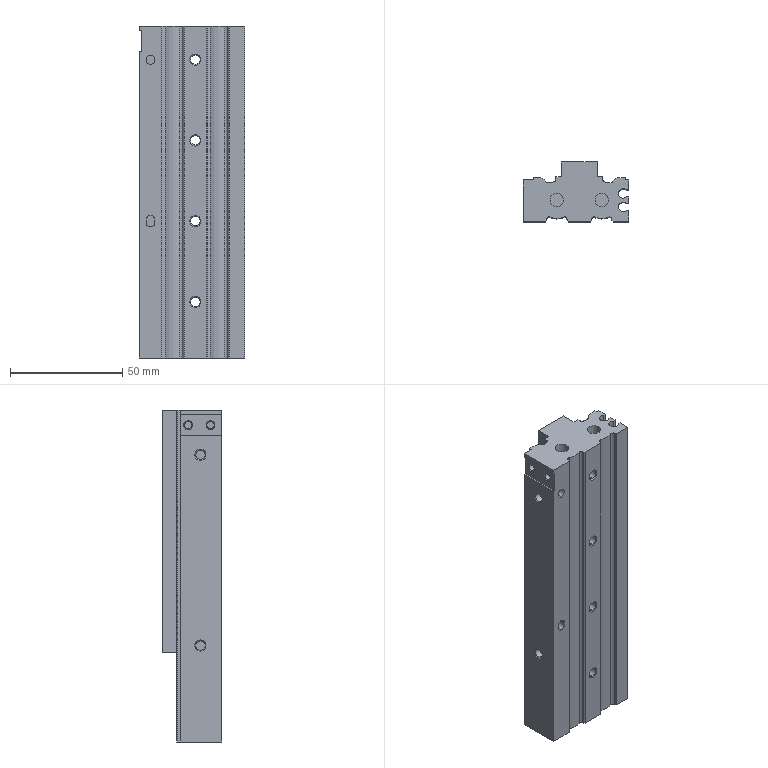Part | SolidWorks | features BaseBody 1 | 1 solid | 152 faces | box 47 x 26.5 x 148 mm | volume 111370 mm3 | cylinder 65 | plane 63 | cone 24 | commonest cylinder face diameters 3.242 x12 4.2 x12 4 x7 2 x6 8.5 x6 4.134 x4